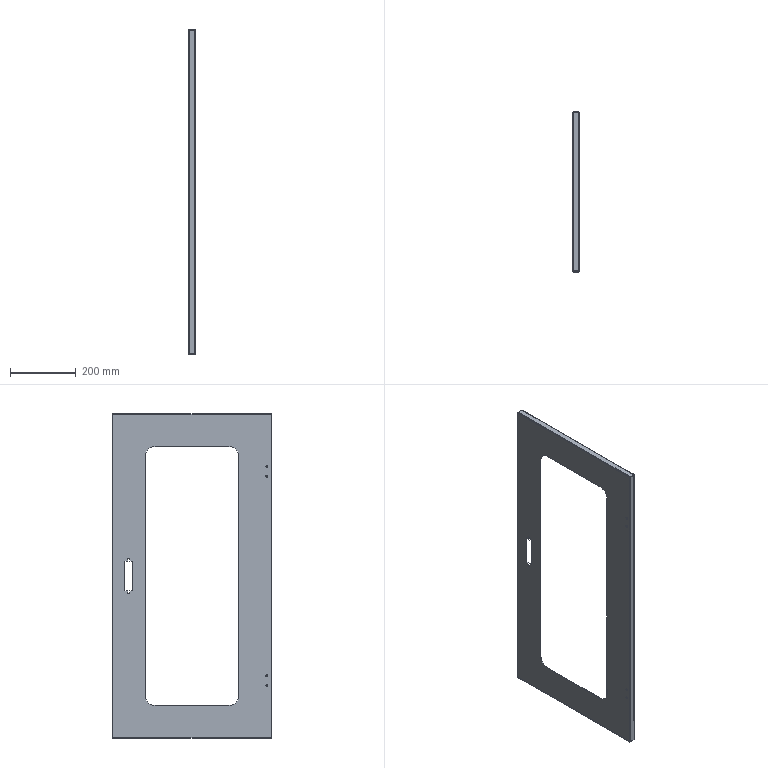Part | STEP file | JBJ-P-1000-13 | 1 solid | 98 faces | box 20 x 485 x 988 mm | volume 412527 mm3 | plane 52 | cylinder 30 | spline 16 | commonest cylinder face diameters 2 x8 4.4 x8 4 x4 6 x4 60 x4 7 x2